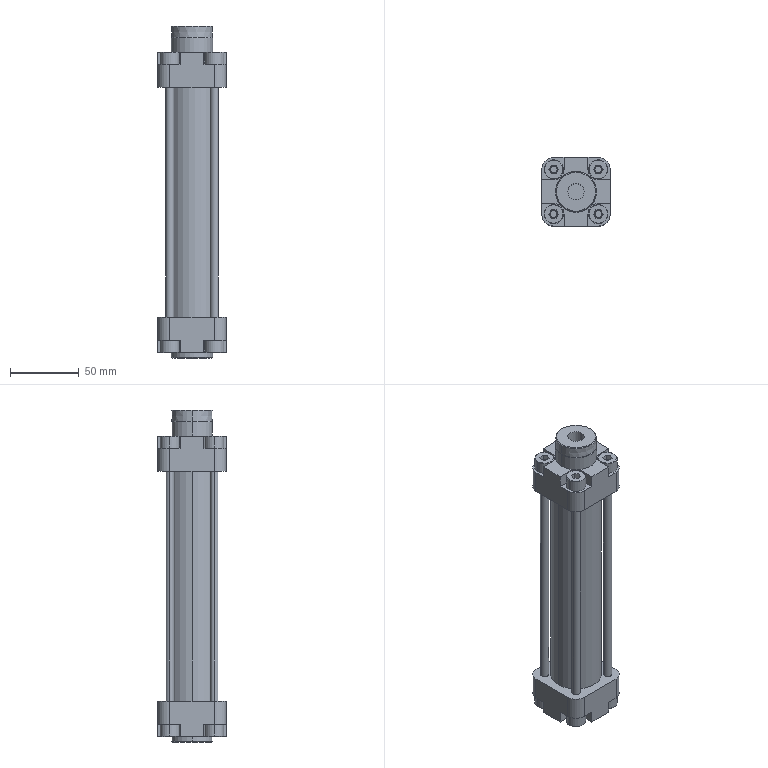Part | STEP file | 1 solid | 306 faces | box 50 x 50 x 242 mm | volume 216779 mm3 | plane 168 | cylinder 86 | cone 36 | torus 16 | commonest cylinder face diameters 4.917 x16 14 x16 6 x12 15.05 x8 17.5 x8 5.9 x4